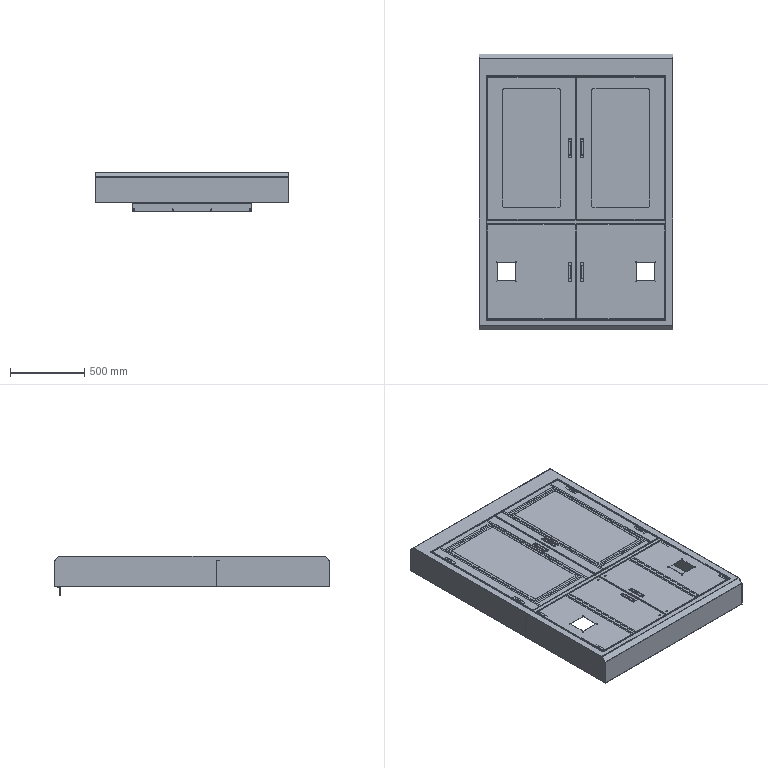Part | NX | features BREP 30 | 63 solids | 2640 faces | box 1300 x 1853 x 268 mm | volume 11251718 mm3 | plane 1262 | cylinder 914 | torus 232 | cone 152 | spline 80 | commonest cylinder face diameters 7 x159 6 x130 4 x95 5 x80 8 x58 10 x48